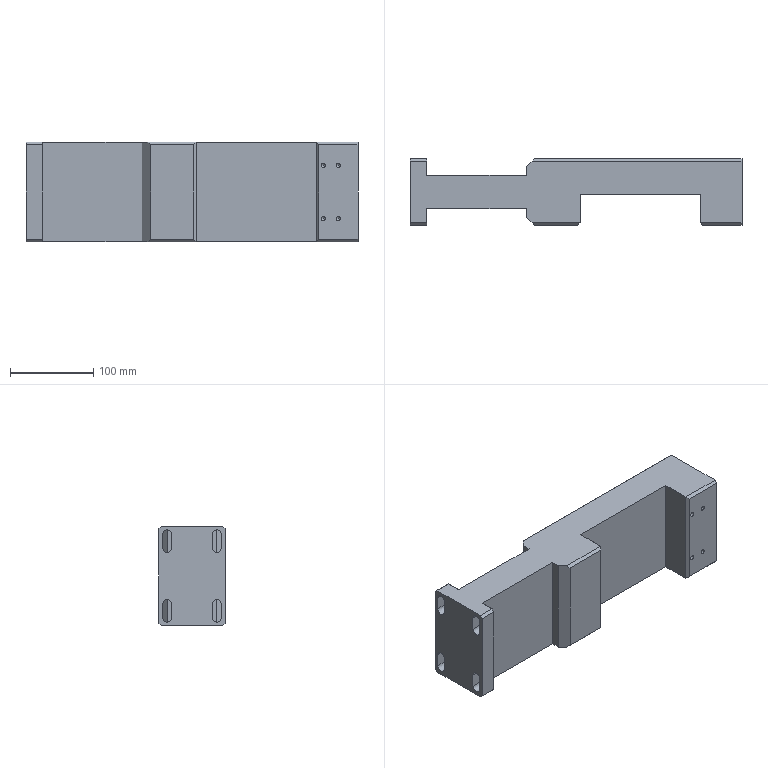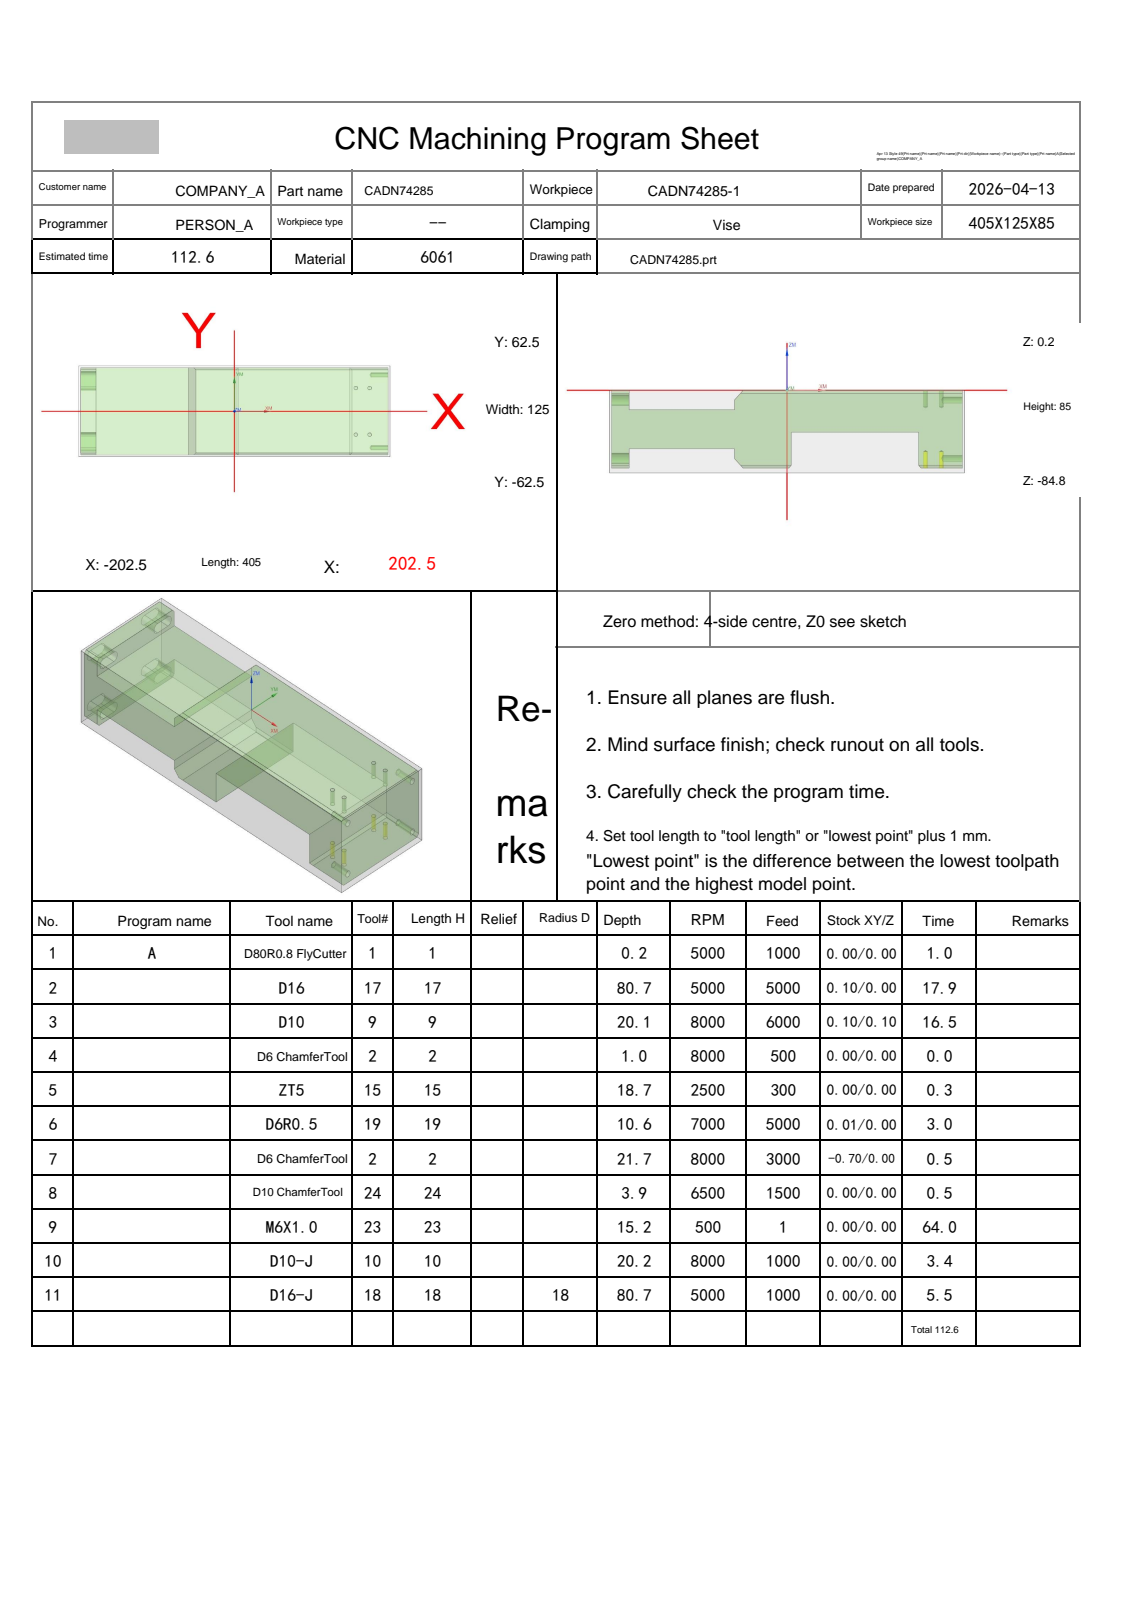NC program | NX | posted by the shop | part box 400 x 80 x 120 mm
Lines 7019 to 8047 of 8047:
N4 T02 M06
(D6 ChamferTool  D=6. R=0. H=02 ce=0.00 di=0.10)
G00 G90 G54 X158. Y-32. M03 S8000
G43 H02 Z20.
M08
G98 G81 X158. Y-32. Z-.8 R1. F500.
X176.
Y32.
X158.
G80
G00 Z20.
G91 G28 Z0.0
M05
M09
G91 G28 Z0.0
M01
N5 T15 M06
(ZT5 D=5. DR_a=118 H=15)
G00 G90 G54 X158. Y-32. M03 S2500
G43 H15 Z20.
M08
G98 G83 X158. Y-32. Z-18.502 R1. F300. Q3.
X176.
Y32.
X158.
G80
G00 Z20.
G91 G28 Z0.0
M05
M09
G91 G28 Z0.0
M01
N6 T19 M06
(D6R0.5  D=6. R=0.5 H=19 ce=0.01 di=0.00)
G00 G90 G54 X-52.801 Y-63.373 M03 S7000
G43 H19 Z10.788
M08
Z.415
G01 Z-.085 F5000.
Y-58.246
Y58.246
X-52.884 Y58.332 Z-.17
X-52.887 Y58.275
Y-58.275
X-52.884 Y-58.332
X-52.968 Y-58.417 Z-.255
X-52.972 Y-58.275
Y58.275
X-52.968 Y58.417
X-53.053 Y58.503 Z-.339
X-53.057 Y58.275
Y-58.275
X-53.053 Y-58.503
X-53.14 Y-58.588 Z-.424
X-53.141 Y-57.278
Y57.278
X-53.14 Y58.588
X-53.224 Y58.674 Z-.509
X-53.226 Y58.622
Y-58.622
X-53.224 Y-58.674
X-53.308 Y-58.759 Z-.594
X-53.311 Y-58.622
Y58.622
X-53.308 Y58.759
X-53.393 Y58.845 Z-.679
X-53.396 Y58.622
Y-58.622
X-53.393 Y-58.844
X-53.479 Y-58.93 Z-.764
X-53.481 Y-57.617
Y57.617
X-53.479 Y58.93
X-53.563 Y59.015 Z-.849
X-53.566 Y58.969
Y-58.969
X-53.563 Y-59.015
X-53.647 Y-59.099 Z-.933
X-53.65 Y-58.969
Y58.969
X-53.647 Y59.099
X-53.732 Y59.184 Z-1.018
X-53.735 Y58.969
Y-58.969
X-53.732 Y-59.184
X-53.819 Y-59.269 Z-1.103
X-53.82 Y-57.957
Y57.957
X-53.819 Y59.269
X-53.903 Y59.354 Z-1.188
X-53.905 Y59.316
Y-59.316
X-53.903 Y-59.354
X-53.987 Y-59.439 Z-1.273
X-53.99 Y-59.316
Y59.316
X-53.987 Y59.439
X-54.071 Y59.523 Z-1.358
X-54.075 Y59.316
Y-59.316
X-54.071 Y-59.523
X-54.158 Y-59.608 Z-1.442
X-54.16 Y-58.296
Y58.296
X-54.158 Y59.608
X-54.243 Y59.693 Z-1.527
X-54.244 Y59.663
Y-59.663
X-54.243 Y-59.693
X-54.326 Y-59.777 Z-1.612
X-54.329 Y-59.663
Y59.663
X-54.326 Y59.778
X-54.411 Y59.862 Z-1.697
X-54.414 Y59.663
Y-59.663
X-54.411 Y-59.862
X-54.497 Y-59.946 Z-1.782
X-54.499 Y-58.635
Y58.635
X-54.497 Y59.946
X-54.583 Y60.03 Z-1.867
X-54.584 Y58.72
Y-58.72
X-54.583 Y-60.03
X-54.666 Y-60.114 Z-1.952
X-54.669 Y-60.009
Y60.009
X-54.666 Y60.114
X-54.75 Y60.198 Z-2.036
X-54.754 Y60.009
Y-60.009
X-54.75 Y-60.198
X-54.836 Y-60.282 Z-2.121
X-54.838 Y-58.975
Y58.975
X-54.836 Y60.282
X-54.923 Y60.366 Z-2.206
Y59.06
Y-59.06
Y-60.366
X-55.005 Y-60.45 Z-2.291
X-55.008 Y-60.356
Y60.356
X-55.005 Y60.45
X-55.089 Y60.534 Z-2.376
X-55.093 Y60.356
Y-60.356
X-55.089 Y-60.534
X-55.175 Y-60.618 Z-2.461
X-55.178 Y-59.314
Y59.314
X-55.175 Y60.618
X-55.263 Y60.703 Z-2.546
Y59.399
Y-59.399
Y-60.703
X-55.346 Y-60.787 Z-2.63
X-55.348 Y-60.703
Y60.703
X-55.346 Y60.787
X-55.429 Y60.87 Z-2.715
X-55.432 Y60.703
Y-60.703
X-55.429 Y-60.87
X-55.514 Y-60.954 Z-2.8
X-55.517 Y-60.703
Y60.703
X-55.514 Y60.954
X-55.602 Y61.038 Z-2.885
Y59.739
Y-59.739
Y-61.038
X-55.645 Y-61.05 Z-2.927
X-55.686 Y-61.061 Z-2.97
X-55.687 Y-59.823
Y59.823
X-55.686 Y61.061
X-55.729 Y61.062 Z-3.012
X-55.771 Z-3.055
X-55.772 Y59.908
Y-59.908
X-55.771 Y-61.063
X-55.814 Z-3.097
X-55.856 Z-3.14
X-55.857 Y-59.993
Y59.993
X-55.856 Y61.063
X-55.899 Y61.064 Z-3.182
X-55.941 Z-3.224
X-55.942 Y60.
Y-60.
X-55.941 Y-61.064
X-55.984 Y-61.065 Z-3.267
X-56.026 Z-3.309
Y-60.
Y60.
Y61.065
X-56.069 Y61.066 Z-3.352
X-56.11 Z-3.394
X-56.111 Y60.
Y-60.
X-56.11 Y-61.066
X-56.154 Z-3.437
X-56.195 Y-61.067 Z-3.479
X-56.196 Y-60.
Y60.
X-56.195 Y61.067
X-56.238 Z-3.521
X-56.28 Y61.068 Z-3.564
X-56.281 Y60.
Y-60.
X-56.28 Y-61.068
X-56.323 Z-3.606
X-56.365 Y-61.069 Z-3.649
X-56.366 Y-60.
Y60.
X-56.365 Y61.069
X-56.408 Z-3.691
X-56.45 Z-3.734
X-56.451 Y60.
Y-60.
X-56.45 Y-61.069
X-56.493 Y-61.07 Z-3.776
X-56.534 Z-3.818
X-56.535 Y-60.
Y60.
X-56.534 Y61.07
X-56.578 Y61.071 Z-3.861
X-56.619 Z-3.903
X-56.62 Y60.
Y-60.
X-56.619 Y-61.071
X-56.663 Y-61.072 Z-3.946
X-56.704 Z-3.988
X-56.705 Y-60.
Y60.
X-56.704 Y61.072
X-56.748 Y61.073 Z-4.031
X-56.789 Z-4.073
X-56.79 Y60.
Y-60.
X-56.789 Y-61.073
X-56.832 Y-61.074 Z-4.115
X-56.874 Z-4.158
X-56.875 Y-60.
Y60.
X-56.874 Y61.074
X-56.917 Z-4.2
X-56.958 Y61.075 Z-4.243
X-56.96 Y61.05
Y-61.05
X-56.958 Y-61.075
X-57.002 Z-4.285
X-57.043 Y-61.076 Z-4.327
X-57.045 Y-61.05
Y61.05
X-57.043 Y61.076
X-57.087 Z-4.37
X-57.128 Y61.077 Z-4.412
X-57.129 Y61.05
Y-61.05
X-57.128 Y-61.077
X-57.172 Z-4.455
X-57.211 Z-4.497
X-57.212 Y-61.05
Y61.05
X-57.211 Y61.077
X-57.257 Y61.078 Z-4.54
X-57.298 Z-4.582
X-57.299 Y61.05
Y-61.05
X-57.298 Y-61.078
X-57.342 Z-4.624
X-57.383 Y-61.079 Z-4.667
X-57.384 Y-61.05
Y61.05
X-57.383 Y61.079
X-57.426 Z-4.709
X-57.467 Z-4.752
X-57.469 Y61.05
Y-61.05
X-57.467 Y-61.079
X-57.511 Z-4.794
X-57.552 Y-61.08 Z-4.837
X-57.554 Y-61.05
Y61.05
X-57.552 Y61.08
X-57.596 Z-4.879
X-57.637 Z-4.921
X-57.639 Y61.05
Y-61.05
X-57.637 Y-61.08
X-57.681 Z-4.964
X-57.722 Y-61.081 Z-5.006
X-57.723 Y-61.05
Y61.05
X-57.722 Y61.081
X-57.766 Z-5.049
X-57.807 Z-5.091
X-57.808 Y61.05
Y-61.05
X-57.807 Y-61.081
X-57.851 Y-61.082 Z-5.134
X-57.892 Z-5.176
X-57.893 Y-61.05
Y61.05
X-57.892 Y61.082
X-57.936 Z-5.218
X-57.976 Z-5.261
X-57.978 Y61.05
Y-61.05
X-57.976 Y-61.082
X-58.02 Y-61.083 Z-5.303
X-58.061 Z-5.346
X-58.063 Y-61.05
Y61.05
X-58.061 Y61.083
X-58.105 Z-5.388
X-58.146 Z-5.431
X-58.148 Y61.05
Y-61.05
X-58.146 Y-61.084
X-58.19 Z-5.473
X-58.231 Z-5.515
X-58.233 Y-61.05
Y61.05
X-58.231 Y61.084
X-58.275 Z-5.558
X-58.316 Y61.085 Z-5.6
X-58.317 Y61.05
Y-61.05
X-58.316 Y-61.085
X-58.36 Z-5.643
X-58.401 Z-5.685
X-58.402 Y-61.05
Y61.05
X-58.401 Y61.085
X-58.445 Z-5.728
X-58.485 Y61.086 Z-5.77
X-58.487 Y61.05
Y-61.05
X-58.485 Y-61.085
X-58.53 Y-61.086 Z-5.812
X-58.57 Z-5.855
X-58.572 Y-61.05
Y61.05
X-58.57 Y61.086
X-58.614 Z-5.897
X-58.655 Z-5.94
X-58.657 Y61.05
Y-61.05
X-58.655 Y-61.086
X-58.699 Z-5.982
X-58.74 Z-6.025
X-58.742 Y-61.05
Y61.05
X-58.74 Y61.086
X-58.784 Z-6.067
X-58.825 Y61.087 Z-6.109
X-58.827 Y61.05
Y-61.05
X-58.825 Y-61.086
X-58.869 Z-6.152
X-58.91 Z-6.194
X-58.911 Y-61.05
Y61.05
X-58.91 Y61.087
X-58.954 Z-6.237
X-58.994 Z-6.279
X-58.996 Y61.05
Y-61.05
X-58.994 Y-61.086
X-59.039 Z-6.322
X-59.079 Z-6.364
X-59.081 Y-61.05
Y61.05
X-59.079 Y61.087
X-59.123 Z-6.406
X-59.164 Z-6.449
X-59.166 Y61.05
Y-61.05
X-59.164 Y-61.086
X-59.208 Z-6.491
X-59.249 Z-6.534
X-59.251 Y-61.05
Y61.05
X-59.249 Y61.087
X-59.293 Z-6.576
X-59.334 Z-6.619
X-59.336 Y61.05
Y-61.05
X-59.334 Y-61.086
X-59.378 Z-6.661
X-59.419 Z-6.703
X-59.42 Y-61.05
Y61.05
X-59.419 Y61.087
X-59.463 Z-6.746
X-59.504 Z-6.788
X-59.505 Y61.05
Y-61.05
X-59.504 Y-61.086
X-59.548 Z-6.831
X-59.588 Z-6.873
X-59.59 Y-61.05
Y61.05
X-59.588 Y61.087
X-59.633 Z-6.916
X-59.673 Z-6.958
X-59.675 Y61.05
Y-61.05
X-59.673 Y-61.086
X-59.717 Z-7.
X-59.758 Z-7.043
X-59.76 Y-61.05
Y61.05
X-59.758 Y61.087
X-59.802 Z-7.085
X-59.844 Z-7.128
X-59.845 Y60.
Y-60.
X-59.844 Y-61.086
X-59.887 Z-7.17
X-59.928 Z-7.212
X-59.93 Y-61.05
Y61.05
X-59.928 Y61.086
X-59.972 Z-7.255
X-60.013 Z-7.297
X-60.014 Y61.05
Y-61.05
X-60.013 Y-61.086
X-60.057 Z-7.34
X-60.098 Z-7.382
X-60.099 Y-61.05
Y61.05
X-60.098 Y61.086
X-60.142 Y61.085 Z-7.425
X-60.182 Z-7.467
X-60.184 Y61.05
Y-61.05
X-60.182 Y-61.085
X-60.227 Z-7.509
X-60.267 Z-7.552
X-60.269 Y-61.05
Y61.05
X-60.267 Y61.085
X-60.311 Z-7.594
X-60.352 Y61.084 Z-7.637
X-60.354 Y61.05
Y-61.05
X-60.352 Y-61.084
X-60.396 Z-7.679
X-60.437 Z-7.722
X-60.439 Y-61.05
Y61.05
X-60.437 Y61.084
X-60.481 Z-7.764
X-60.522 Y61.083 Z-7.806
X-60.524 Y61.05
Y-61.05
X-60.522 Y-61.083
X-60.566 Z-7.849
X-60.607 Z-7.891
X-60.608 Y-61.05
Y61.05
X-60.607 Y61.083
X-60.651 Y61.082 Z-7.934
X-60.692 Z-7.976
X-60.693 Y61.05
Y-61.05
X-60.692 Y-61.082
X-60.736 Z-8.019
X-60.777 Z-8.061
X-60.778 Y-61.05
Y61.05
X-60.777 Y61.082
X-60.821 Y61.081 Z-8.103
X-60.861 Z-8.146
X-60.863 Y61.05
Y-61.05
X-60.861 Y-61.081
X-60.905 Z-8.188
X-60.946 Z-8.231
X-60.948 Y-61.05
Y61.05
X-60.946 Y61.08
X-60.99 Z-8.273
X-61.031 Z-8.316
X-61.033 Y61.05
Y-61.05
X-61.031 Y-61.08
X-61.075 Z-8.358
X-61.116 Z-8.4
X-61.118 Y-61.05
Y61.05
X-61.116 Y61.079
X-61.16 Z-8.443
X-61.201 Z-8.485
X-61.202 Y61.05
Y-61.05
X-61.201 Y-61.079
X-61.245 Z-8.528
X-61.286 Y-61.078 Z-8.57
X-61.287 Y-61.05
Y61.05
X-61.286 Y61.078
X-61.33 Z-8.613
X-61.371 Z-8.655
X-61.372 Y61.05
Y-61.05
X-61.371 Y-61.078
X-61.415 Y-61.077 Z-8.697
X-61.456 Z-8.74
X-61.457 Y-61.05
Y61.05
X-61.456 Y61.077
X-61.499 Y61.076 Z-8.782
X-61.54 Z-8.825
X-61.542 Y61.05
Y-61.05
X-61.54 Y-61.076
X-61.584 Z-8.867
X-61.625 Y-61.075 Z-8.91
X-61.627 Y-61.05
Y61.05
X-61.625 Y61.075
X-61.669 Z-8.952
X-61.71 Y61.074 Z-8.994
X-61.712 Y60.
Y-60.
X-61.71 Y-61.074
X-61.754 Z-9.037
X-61.795 Y-61.073 Z-9.079
X-61.796 Y-60.
Y60.
X-61.795 Y61.073
X-61.839 Z-9.122
X-61.88 Y61.072 Z-9.164
X-61.881 Y60.
Y-60.
X-61.88 Y-61.073
X-61.924 Y-61.072 Z-9.207
X-61.965 Z-9.249
X-61.966 Y-60.
Y60.
X-61.965 Y61.072
X-62.008 Y61.071 Z-9.291
X-62.05 Z-9.334
X-62.051 Y60.
Y-60.
X-62.05 Y-61.071
X-62.093 Y-61.07 Z-9.376
X-62.135 Z-9.419
X-62.136 Y-60.
Y60.
X-62.135 Y61.07
X-62.178 Z-9.461
X-62.22 Y61.069 Z-9.504
X-62.221 Y60.
Y-60.
X-62.22 Y-61.069
X-62.263 Z-9.546
X-62.304 Y-61.068 Z-9.588
X-62.305 Y-60.
Y60.
X-62.304 Y61.068
X-62.348 Z-9.631
X-62.389 Y61.067 Z-9.673
X-62.39 Y60.
Y-60.
X-62.389 Y-61.067
X-62.433 Z-9.716
X-62.474 Y-61.066 Z-9.758
X-62.475 Y-60.
Y60.
X-62.474 Y61.066
X-62.518 Z-9.801
X-62.559 Z-9.843
X-62.56 Y60.
Y-60.
X-62.559 Y-61.066
X-62.602 Y-61.065 Z-9.885
X-62.644 Z-9.928
X-62.645 Y-60.
Y60.
X-62.644 Y61.065
X-62.687 Y61.064 Z-9.97
X-62.729 Z-10.013
X-62.73 Y60.
Y-60.
X-62.729 Y-61.064
X-62.772 Y-61.063 Z-10.055
X-62.814 Z-10.097
X-62.815 Y-59.949
Y59.949
X-62.814 Y61.063
X-62.852 Y61.062 Z-10.135
X-62.89 Z-10.173
Y-61.062
X-62.928 Y-61.061 Z-10.211
X-62.965 Y-61.06 Z-10.249
Y61.06
X-63.04 Y61.022 Z-10.324
Y-61.022
X-63.114 Y-60.947 Z-10.4
Y60.947
G00 Z10.788
G91 G28 Z0.0
M05
M09
G91 G28 Z0.0
M01
N7 T02 M06
(D6 ChamferTool  D=6. R=0. H=02 ce=0.00 di=0.00)
G00 G90 G54 X-178.793 Y57.461 M03 S8000
G43 H02 Z20.
M08
Z2.935
G01 Z-1.5 F3000.
X-178.733 Y57.289
X-178.7 Y57.
Y-57.
X-178.733 Y-57.289
X-178.793 Y-57.461
Z2.935
G00 Z20.
X-201.207
Z2.935
G01 Z-1.5
X-201.267 Y-57.289
X-201.3 Y-57.
Y0.0
Y57.
X-201.267 Y57.289
X-201.207 Y57.461
Z2.935
G00 Z20.
X201.207
Z2.935
G01 Z-1.5
X201.267 Y57.289
X201.3 Y57.
Y-57.
X201.267 Y-57.289
X201.207 Y-57.461
Z2.935
G00 Z20.
X-62.996 Y-62.128
Z-7.148
G01 Z-21.5
G03 X-62.915 Y-61.828 I-.52 J.3
X-63.215 Y-61.308 I-.6 J0.0
G01 X-63.245 Y-61.3
X-176.755
X-176.785 Y-61.308
G03 X-177.085 Y-61.828 I.3 J-.52
X-177.004 Y-62.128 I.6 J0.0
G01 Z-.177
G00 Z20.
Y62.128
Z-.177
G01 Z-21.5
G03 X-177.085 Y61.828 I.52 J-.3
X-176.785 Y61.308 I.6 J0.0
G01 X-176.755 Y61.3
X-63.245
X-63.215 Y61.308
G03 X-62.915 Y61.828 I-.3 J.52
X-62.996 Y62.128 I-.6 J0.0
G01 Z-7.148
G00 Z20.
G00 G90 X157.13 Y-32.232 M03 S8000
Z20.
Z-.8
G01 Z-1.3 F600.
X156.5 Y-32.4
G03 X158. Y-33.9 I1.5 J0.0
X159.9 Y-32. I0.0 J1.9
X158. Y-30.1 I-1.9 J0.0
X156.1 Y-32. I0.0 J-1.9
X158. Y-33.9 I1.9 J0.0
X159.5 Y-32.4 I0.0 J1.5
G01 X158.87 Y-32.232
Z-.8
G00 Z20.
X175.13
Z-.8
G01 Z-1.3
X174.5 Y-32.4
G03 X176. Y-33.9 I1.5 J0.0
X177.9 Y-32. I0.0 J1.9
X176. Y-30.1 I-1.9 J0.0
X174.1 Y-32. I0.0 J-1.9
X176. Y-33.9 I1.9 J0.0
X177.5 Y-32.4 I0.0 J1.5
G01 X176.87 Y-32.232
Z-.8
G00 Z20.
X175.13 Y31.768
Z-.8
G01 Z-1.3
X174.5 Y31.6
G03 X176. Y30.1 I1.5 J0.0
X177.9 Y32. I0.0 J1.9
X176. Y33.9 I-1.9 J0.0
X174.1 Y32. I0.0 J-1.9
X176. Y30.1 I1.9 J0.0
X177.5 Y31.6 I0.0 J1.5
G01 X176.87 Y31.768
Z-.8
G00 Z20.
X157.13
Z-.8
G01 Z-1.3
X156.5 Y31.6
G03 X158. Y30.1 I1.5 J0.0
X159.9 Y32. I0.0 J1.9
X158. Y33.9 I-1.9 J0.0
X156.1 Y32. I0.0 J-1.9
X158. Y30.1 I1.9 J0.0
X159.5 Y31.6 I0.0 J1.5
G01 X158.87 Y31.768
Z-.8
G00 Z20.
G91 G28 Z0.0
M05
M09
G91 G28 Z0.0
M01
N8 T24 M06
(D10 ChamferTool  D=10. R=0. H=24 ce=0.00 di=0.00)
G00 G90 G54 X-172.29 Y-62.7 M03 S6500
G43 H24 Z20.
M08
Z-2.2
G01 Z-3.7 F1500.
G03 X-174.29 Y-60.7 I-2. J0.0
G01 X-204.603
G03 X-205.7 Y-61.028 I0.0 J-2.
G01 Z-2.2
G00 Z20.
Y61.028
Z-2.2
G01 Z-3.7
G03 X-204.603 Y60.7 I1.097 J1.672
G01 X-174.29
G03 X-172.29 Y62.7 I0.0 J2.
G01 Z-2.2
G00 Z20.
X-59.603
Z-2.2
G01 Z-3.7
G03 X-57.603 Y60.7 I2. J0.0
G01 X204.603
G03 X205.7 Y61.028 I0.0 J2.
G01 Z-2.2
G00 Z20.
Y-61.028
Z-2.2
G01 Z-3.7
G03 X204.603 Y-60.7 I-1.097 J-1.672
G01 X-57.603
G03 X-59.603 Y-62.7 I0.0 J-2.
G01 Z-2.2
G00 Z20.
G91 G28 Z0.0
M05
M09
G91 G28 Z0.0
M01
N9 T23 M06
(M6X1.0 D=5. DR_a=180 H=23)
G00 G90 G54 X158. Y-32. M03 S500
G43 H23 Z20.
M08
G95
G98 G84 X158. Y-32. Z-15. R1. F1. Q3.
X176.
Y32.
X158.
G80
G94
G00 Z20.
G91 G28 Z0.0
M05
M09
G91 G28 Z0.0
M01
N10 T10 M06
(D10-J  D=10. R=0. H=10 ce=0.40 di=0.00)
G00 G90 G54 X-176.598 Y-67. M03 S8000
G43 H10 Z10.4
M08
Z-18.5
G01 Z-20. F1000.
G03 X-174.599 Y-65. I-.001 J2.
G01 Y64.1
G02 X-173.699 Y65. I.9 J0.0
G01 X-170.635
G02 X-169.635 Y64. I0.0 J-1.
G01 Y-64.1
G03 X-168.735 Y-65. I.9 J0.0
G01 X-165.672
G03 X-164.672 Y-64. I0.0 J1.
G01 Y64.1
G02 X-163.772 Y65. I.9 J0.0
G01 X-160.708
G02 X-159.708 Y64. I0.0 J-1.
G01 Y-64.1
G03 X-158.808 Y-65. I.9 J0.0
G01 X-155.745
G03 X-154.745 Y-64. I0.0 J1.
G01 Y64.1
G02 X-153.845 Y65. I.9 J0.0
G01 X-150.781
G02 X-149.781 Y64. I0.0 J-1.
G01 Y-64.1
G03 X-148.881 Y-65. I.9 J0.0
G01 X-145.817
G03 X-144.817 Y-64. I0.0 J1.
G01 Y64.1
G02 X-143.917 Y65. I.9 J0.0
G01 X-140.854
G02 X-139.854 Y64. I0.0 J-1.
G01 Y-64.1
G03 X-138.954 Y-65. I.9 J0.0
G01 X-135.89
G03 X-134.89 Y-64. I0.0 J1.
G01 Y64.1
G02 X-133.99 Y65. I.9 J0.0
G01 X-130.927
G02 X-129.927 Y64. I0.0 J-1.
G01 Y-64.1
G03 X-129.027 Y-65. I.9 J0.0
G01 X-125.963
G03 X-124.963 Y-64. I0.0 J1.
G01 Y64.
G02 X-123.963 Y65. I1. J0.0
G01 X-120.9
G02 X-120. Y64.1 I0.0 J-.9
G01 Y-64.
G03 X-119. Y-65. I1. J0.0
G01 X-115.936
G03 X-115.036 Y-64.1 I0.0 J.9
G01 Y64.1
G02 X-114.136 Y65. I.9 J0.0
G01 X-111.072
G02 X-110.072 Y64. I0.0 J-1.
G01 Y-64.1
G03 X-109.172 Y-65. I.9 J0.0
G01 X-106.109
G03 X-105.109 Y-64. I0.0 J1.
G01 Y64.1
G02 X-104.209 Y65. I.9 J0.0
G01 X-101.145
G02 X-100.145 Y64. I0.0 J-1.
G01 Y-64.1
G03 X-99.245 Y-65. I.9 J0.0
G01 X-96.182
G03 X-95.182 Y-64. I0.0 J1.
G01 Y64.1
G02 X-94.282 Y65. I.9 J0.0
G01 X-91.218
G02 X-90.218 Y64. I0.0 J-1.
G01 Y-64.1
G03 X-89.318 Y-65. I.9 J0.0
G01 X-86.254
G03 X-85.254 Y-64. I0.0 J1.
G01 Y64.1
G02 X-84.354 Y65. I.9 J0.0
G01 X-81.291
G02 X-80.291 Y64. I0.0 J-1.
G01 Y-64.1
G03 X-79.391 Y-65. I.9 J0.0
G01 X-76.327
G03 X-75.327 Y-64. I0.0 J1.
G01 Y64.1
G02 X-74.427 Y65. I.9 J0.0
G01 X-71.364
G02 X-70.364 Y64. I0.0 J-1.
G01 Y-64.1
G03 X-69.464 Y-65. I.9 J0.0
G01 X-66.4
G03 X-65.4 Y-64. I0.0 J1.
G01 Y65.
G03 X-67.399 Y67. I-2. J0.0
G01 Z-18.5
G00 Z10.4
G00 G90 X-178.468 Y67.191 M03 S8000
Z10.2
Z-19.
G01 Z-20. F1000.
G41 D10
X-178.527 Y67.
G03 X-178.615 Y66.414 I1.912 J-.586
X-178.029 Y65. I2. J0.0
G01 X-175. Y61.971
Y-61.971
X-178.029 Y-65.
G03 X-178.615 Y-66.414 I1.414 J-1.414
X-178.527 Y-67. I2. J0.0
G01 G40 X-178.468 Y-67.191
Z-19.
G00 X-61.532
G01 Z-20.
G41 D10
X-61.473 Y-67.
G03 X-61.385 Y-66.414 I-1.912 J.586
X-61.971 Y-65. I-2. J0.0
G01 X-65. Y-61.971
Y61.971
X-61.971 Y65.
G03 X-61.385 Y66.414 I-1.414 J1.414
X-61.473 Y67. I-2. J0.0
G01 G40 X-61.532 Y67.191
Z-19.
G00 Z10.2
G91 G28 Z0.0
M05
M09
G91 G28 Z0.0
M01
N11 T18 M06
(D16-J  D=16. R=0. H=18 ce=0.00 di=0.00)
G00 G90 G54 X201.01 Y-69.144 M03 S5000
G43 H18 Z20.
M08
Z-15.6
G01 Z-16.1 F1000.
G41 D18
X200.998 Y-68.944
G03 X200. Y-68. I-.998 J-.056
G01 X-200.
G02 X-208. Y-60. I0.0 J8.
G01 Y60.
G02 X-200. Y68. I8. J0.0
G01 X200.
G02 X208. Y60. I0.0 J-8.
G01 Y-60.
G02 X200. Y-68. I-8. J0.0
G01 X199.5
G03 X198.5 Y-69. I0.0 J-1.
G01 G40 Y-69.2
Z-15.6
G00 Z20.
X201.01 Y-69.144
Z-31.7
G01 Z-32.2
G41 D18
X200.998 Y-68.944
G03 X200. Y-68. I-.998 J-.056
G01 X-200.
G02 X-208. Y-60. I0.0 J8.
G01 Y60.
G02 X-200. Y68. I8. J0.0
G01 X200.
G02 X208. Y60. I0.0 J-8.
G01 Y-60.
G02 X200. Y-68. I-8. J0.0
G01 X199.5
G03 X198.5 Y-69. I0.0 J-1.
G01 G40 Y-69.2
Z-31.7
G00 Z20.
X201.01 Y-69.144
Z-47.8
G01 Z-48.3
G41 D18
X200.998 Y-68.944
G03 X200. Y-68. I-.998 J-.056
G01 X-200.
G02 X-208. Y-60. I0.0 J8.
G01 Y60.
G02 X-200. Y68. I8. J0.0
G01 X200.
G02 X208. Y60. I0.0 J-8.
G01 Y-60.
G02 X200. Y-68. I-8. J0.0
G01 X199.5
G03 X198.5 Y-69. I0.0 J-1.
G01 G40 Y-69.2
Z-47.8
G00 Z20.
X201.01 Y-69.144
Z-63.9
G01 Z-64.4
G41 D18
X200.998 Y-68.944
G03 X200. Y-68. I-.998 J-.056
G01 X-200.
G02 X-208. Y-60. I0.0 J8.
G01 Y60.
G02 X-200. Y68. I8. J0.0
G01 X200.
G02 X208. Y60. I0.0 J-8.
G01 Y-60.
G02 X200. Y-68. I-8. J0.0
G01 X199.5
G03 X198.5 Y-69. I0.0 J-1.
G01 G40 Y-69.2
Z-63.9
G00 Z20.
X201.01 Y-69.144
Z-80.
G01 Z-80.5
G41 D18
X200.998 Y-68.944
G03 X200. Y-68. I-.998 J-.056
G01 X-200.
G02 X-208. Y-60. I0.0 J8.
G01 Y60.
G02 X-200. Y68. I8. J0.0
G01 X200.
G02 X208. Y60. I0.0 J-8.
G01 Y-60.
G02 X200. Y-68. I-8. J0.0
G01 X199.5
G03 X198.5 Y-69. I0.0 J-1.
G01 G40 Y-69.2
Z-80.
G00 Z20.
M05
M09
G91 G28 Z0.0
G91 G28 Y0.0
M30
%